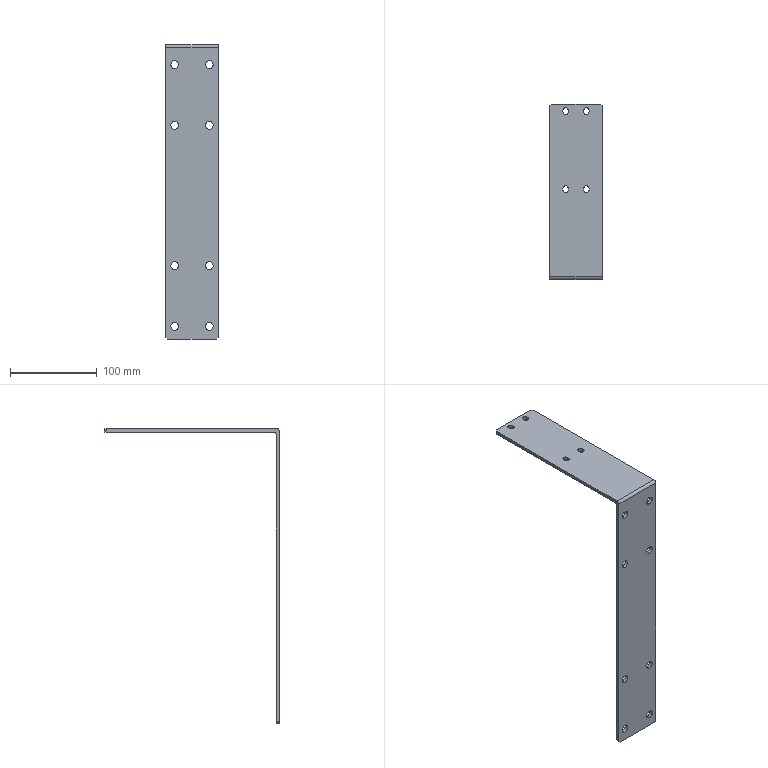Part | STEP file | Cable Carrier Bracket | 1 solid | 46 faces | box 60 x 202 x 340 mm | volume 126408 mm3 | cylinder 26 | plane 20 | commonest cylinder face diameters 9 x16 6 x10